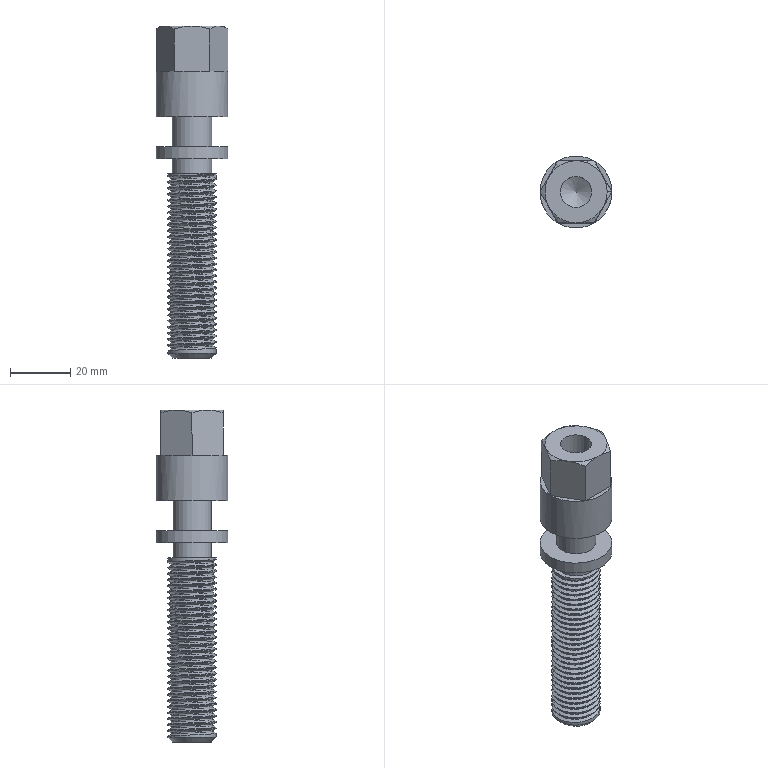Part | NX | features CYLINDER 5, DATUM_CSYS 4, SKETCH 3, SKIN 2, CHAMFER 1, DATUM_ON_PATH 1, DATUM_PLANE 1, EXTRUDE 1, HOLE PACKAGE 1, SIMPLE HOLE 1, SYMBOLIC_THREAD 1, THREADS 1, TRIM BODY 1 | 1 solid | 39 faces | box 23.8 x 23.8 x 110 mm | volume 24209 mm3 | plane 20 | spline 10 | cylinder 7 | cone 2 | commonest cylinder face diameters 13 x2 23.8 x2 10.3 x1 14 x1 16 x1